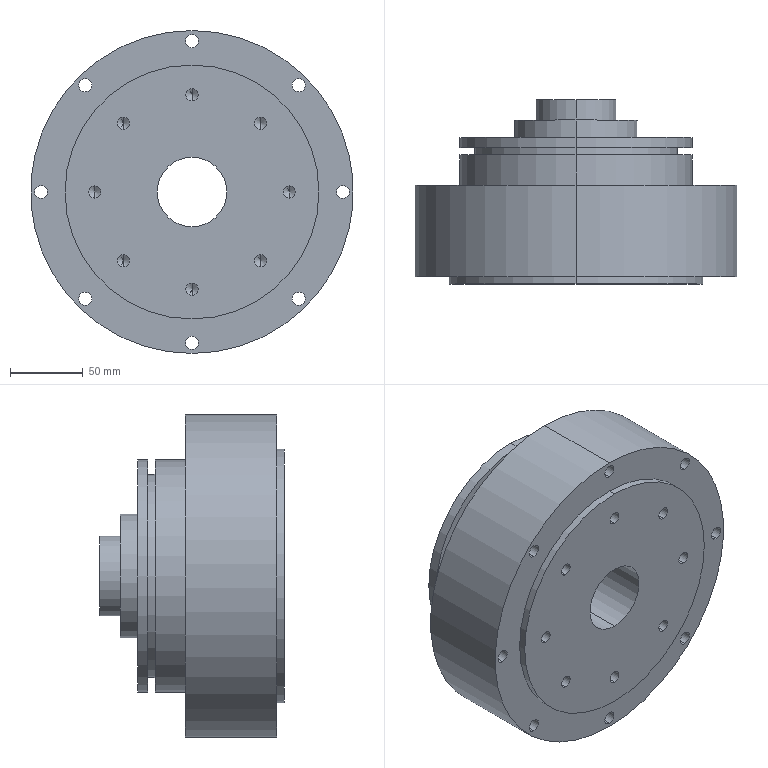Part | SolidWorks | features HoleWzd 2, ICE 1, RevCut 1, Revolution 1 | 1 solid | 72 faces | box 222.5 x 127 x 222.5 mm | volume 3037750 mm3 | cylinder 48 | cone 16 | plane 8 | commonest cylinder face diameters 8.5 x16 9 x16 160 x4 48 x2 55 x2 85 x2